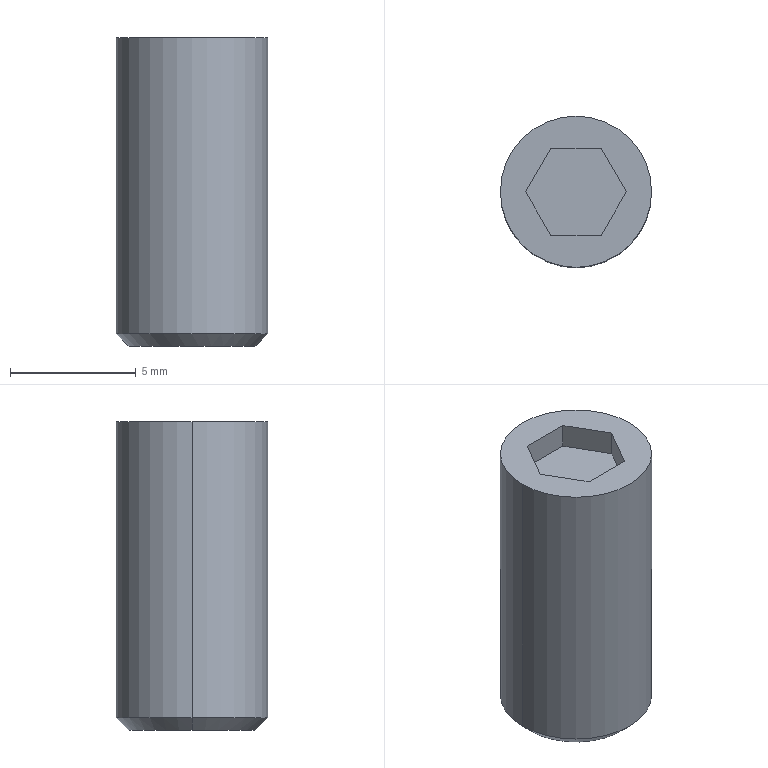Part | SolidWorks | features BaseBody 1 | 1 solid | 13 faces | box 6 x 6 x 12.25 mm | volume 333.743 mm3 | plane 9 | cylinder 2 | cone 2 | commonest cylinder face diameters 6 x2
STEP:
#1=CARTESIAN_POINT('',(24.,133.,18.25));
#2=VERTEX_POINT('',#1);
#3=CARTESIAN_POINT('',(18.,133.,18.25));
#4=VERTEX_POINT('',#3);
#5=CARTESIAN_POINT('',(21.,133.,18.25));
#6=DIRECTION('',(0.,0.,1.));
#7=DIRECTION('',(1.,0.,0.));
#8=AXIS2_PLACEMENT_3D('',#5,#6,#7);
#9=CIRCLE('',#8,3.);
#10=EDGE_CURVE('',#2,#4,#9,.T.);
#11=ORIENTED_EDGE('',*,*,#10,.T.);
#12=CARTESIAN_POINT('',(18.,133.,30.));
#13=VERTEX_POINT('',#12);
#14=CARTESIAN_POINT('',(18.,133.,29.));
#15=DIRECTION('',(0.,0.,1.));
#16=VECTOR('',#15,1000.);
#17=LINE('',#14,#16);
#18=EDGE_CURVE('',#4,#13,#17,.T.);
#19=ORIENTED_EDGE('',*,*,#18,.T.);
#20=CARTESIAN_POINT('',(24.,133.,30.));
#21=VERTEX_POINT('',#20);
#22=CARTESIAN_POINT('',(21.,133.,30.));
#23=DIRECTION('',(0.,0.,-1.));
#24=DIRECTION('',(1.,0.,0.));
#25=AXIS2_PLACEMENT_3D('',#22,#23,#24);
#26=CIRCLE('',#25,3.);
#27=EDGE_CURVE('',#13,#21,#26,.T.);
#28=ORIENTED_EDGE('',*,*,#27,.T.);
#29=CARTESIAN_POINT('',(24.,133.,29.));
#30=DIRECTION('',(0.,0.,1.));
#31=VECTOR('',#30,1000.);
#32=LINE('',#29,#31);
#33=EDGE_CURVE('',#2,#21,#32,.T.);
#34=ORIENTED_EDGE('',*,*,#33,.F.);
#35=EDGE_LOOP('',(#11,#19,#28,#34));
#36=FACE_OUTER_BOUND('',#35,.T.);
#37=CARTESIAN_POINT('',(21.,133.,29.));
#38=DIRECTION('',(0.,0.,1.));
#39=DIRECTION('',(1.,0.,0.));
#40=AXIS2_PLACEMENT_3D('',#37,#38,#39);
#41=CYLINDRICAL_SURFACE('',#40,3.);
#42=ADVANCED_FACE('',(#36),#41,.T.);
#43=CARTESIAN_POINT('',(23.5,133.,17.75));
#44=VERTEX_POINT('',#43);
#45=CARTESIAN_POINT('',(18.5,133.,17.75));
#46=VERTEX_POINT('',#45);
#47=CARTESIAN_POINT('',(21.,133.,17.75));
#48=DIRECTION('',(0.,0.,1.));
#49=DIRECTION('',(1.,0.,0.));
#50=AXIS2_PLACEMENT_3D('',#47,#48,#49);
#51=CIRCLE('',#50,2.5);
#52=EDGE_CURVE('',#44,#46,#51,.T.);
#53=ORIENTED_EDGE('',*,*,#52,.T.);
#54=CARTESIAN_POINT('',(18.,133.,18.25));
#55=DIRECTION('',(-0.7071,0.,0.7071));
#56=VECTOR('',#55,1000.);
#57=LINE('',#54,#56);
#58=EDGE_CURVE('',#46,#4,#57,.T.);
#59=ORIENTED_EDGE('',*,*,#58,.T.);
#60=ORIENTED_EDGE('',*,*,#10,.F.);
#61=CARTESIAN_POINT('',(24.,133.,18.25));
#62=DIRECTION('',(0.7071,0.,0.7071));
#63=VECTOR('',#62,1000.);
#64=LINE('',#61,#63);
#65=EDGE_CURVE('',#44,#2,#64,.T.);
#66=ORIENTED_EDGE('',*,*,#65,.F.);
#67=EDGE_LOOP('',(#53,#59,#60,#66));
#68=FACE_OUTER_BOUND('',#67,.T.);
#69=CARTESIAN_POINT('',(21.,133.,18.25));
#70=DIRECTION('',(0.,0.,1.));
#71=DIRECTION('',(1.,0.,0.));
#72=AXIS2_PLACEMENT_3D('',#69,#70,#71);
#73=CONICAL_SURFACE('',#72,3.,0.7854);
#74=ADVANCED_FACE('',(#68),#73,.T.);
#75=ORIENTED_EDGE('',*,*,#18,.F.);
#76=CARTESIAN_POINT('',(21.,133.,18.25));
#77=DIRECTION('',(0.,0.,1.));
#78=DIRECTION('',(1.,0.,0.));
#79=AXIS2_PLACEMENT_3D('',#76,#77,#78);
#80=CIRCLE('',#79,3.);
#81=EDGE_CURVE('',#4,#2,#80,.T.);
#82=ORIENTED_EDGE('',*,*,#81,.T.);
#83=ORIENTED_EDGE('',*,*,#33,.T.);
#84=CARTESIAN_POINT('',(21.,133.,30.));
#85=DIRECTION('',(0.,0.,-1.));
#86=DIRECTION('',(1.,0.,0.));
#87=AXIS2_PLACEMENT_3D('',#84,#85,#86);
#88=CIRCLE('',#87,3.);
#89=EDGE_CURVE('',#21,#13,#88,.T.);
#90=ORIENTED_EDGE('',*,*,#89,.T.);
#91=EDGE_LOOP('',(#75,#82,#83,#90));
#92=FACE_OUTER_BOUND('',#91,.T.);
#93=CARTESIAN_POINT('',(21.,133.,29.));
#94=DIRECTION('',(0.,0.,1.));
#95=DIRECTION('',(1.,0.,0.));
#96=AXIS2_PLACEMENT_3D('',#93,#94,#95);
#97=CYLINDRICAL_SURFACE('',#96,3.);
#98=ADVANCED_FACE('',(#92),#97,.T.);
#99=ORIENTED_EDGE('',*,*,#89,.F.);
#100=ORIENTED_EDGE('',*,*,#27,.F.);
#101=EDGE_LOOP('',(#99,#100));
#102=FACE_OUTER_BOUND('',#101,.T.);
#103=CARTESIAN_POINT('',(19.,133.,30.));
#104=VERTEX_POINT('',#103);
#105=CARTESIAN_POINT('',(20.,134.732,30.));
#106=VERTEX_POINT('',#105);
#107=CARTESIAN_POINT('',(19.,133.,30.));
#108=DIRECTION('',(0.5,0.866,0.));
#109=VECTOR('',#108,1000.);
#110=LINE('',#107,#109);
#111=EDGE_CURVE('',#104,#106,#110,.T.);
#112=ORIENTED_EDGE('',*,*,#111,.T.);
#113=CARTESIAN_POINT('',(22.,134.732,30.));
#114=VERTEX_POINT('',#113);
#115=CARTESIAN_POINT('',(33.,134.732,30.));
#116=DIRECTION('',(1.,0.,0.));
#117=VECTOR('',#116,1000.);
#118=LINE('',#115,#117);
#119=EDGE_CURVE('',#106,#114,#118,.T.);
#120=ORIENTED_EDGE('',*,*,#119,.T.);
#121=CARTESIAN_POINT('',(23.,133.,30.));
#122=VERTEX_POINT('',#121);
#123=CARTESIAN_POINT('',(22.,134.732,30.));
#124=DIRECTION('',(0.5,-0.866,0.));
#125=VECTOR('',#124,1000.);
#126=LINE('',#123,#125);
#127=EDGE_CURVE('',#114,#122,#126,.T.);
#128=ORIENTED_EDGE('',*,*,#127,.T.);
#129=CARTESIAN_POINT('',(22.,131.268,30.));
#130=VERTEX_POINT('',#129);
#131=CARTESIAN_POINT('',(23.,133.,30.));
#132=DIRECTION('',(-0.5,-0.866,0.));
#133=VECTOR('',#132,1000.);
#134=LINE('',#131,#133);
#135=EDGE_CURVE('',#122,#130,#134,.T.);
#136=ORIENTED_EDGE('',*,*,#135,.T.);
#137=CARTESIAN_POINT('',(20.,131.268,30.));
#138=VERTEX_POINT('',#137);
#139=CARTESIAN_POINT('',(33.,131.268,30.));
#140=DIRECTION('',(-1.,0.,0.));
#141=VECTOR('',#140,1000.);
#142=LINE('',#139,#141);
#143=EDGE_CURVE('',#130,#138,#142,.T.);
#144=ORIENTED_EDGE('',*,*,#143,.T.);
#145=CARTESIAN_POINT('',(20.,131.268,30.));
#146=DIRECTION('',(-0.5,0.866,0.));
#147=VECTOR('',#146,1000.);
#148=LINE('',#145,#147);
#149=EDGE_CURVE('',#138,#104,#148,.T.);
#150=ORIENTED_EDGE('',*,*,#149,.T.);
#151=EDGE_LOOP('',(#112,#120,#128,#136,#144,#150));
#152=FACE_BOUND('',#151,.T.);
#153=CARTESIAN_POINT('',(33.,108.75,30.));
#154=DIRECTION('',(0.,0.,1.));
#155=DIRECTION('',(1.,0.,0.));
#156=AXIS2_PLACEMENT_3D('',#153,#154,#155);
#157=PLANE('',#156);
#158=ADVANCED_FACE('',(#102,#152),#157,.T.);
#159=ORIENTED_EDGE('',*,*,#58,.F.);
#160=CARTESIAN_POINT('',(21.,133.,17.75));
#161=DIRECTION('',(0.,0.,1.));
#162=DIRECTION('',(1.,0.,0.));
#163=AXIS2_PLACEMENT_3D('',#160,#161,#162);
#164=CIRCLE('',#163,2.5);
#165=EDGE_CURVE('',#46,#44,#164,.T.);
#166=ORIENTED_EDGE('',*,*,#165,.T.);
#167=ORIENTED_EDGE('',*,*,#65,.T.);
#168=ORIENTED_EDGE('',*,*,#81,.F.);
#169=EDGE_LOOP('',(#159,#166,#167,#168));
#170=FACE_OUTER_BOUND('',#169,.T.);
#171=CARTESIAN_POINT('',(21.,133.,18.25));
#172=DIRECTION('',(0.,0.,1.));
#173=DIRECTION('',(1.,0.,0.));
#174=AXIS2_PLACEMENT_3D('',#171,#172,#173);
#175=CONICAL_SURFACE('',#174,3.,0.7854);
#176=ADVANCED_FACE('',(#170),#175,.T.);
#177=ORIENTED_EDGE('',*,*,#119,.F.);
#178=CARTESIAN_POINT('',(20.,134.732,29.));
#179=VERTEX_POINT('',#178);
#180=CARTESIAN_POINT('',(20.,134.732,30.));
#181=DIRECTION('',(0.,0.,-1.));
#182=VECTOR('',#181,1000.);
#183=LINE('',#180,#182);
#184=EDGE_CURVE('',#106,#179,#183,.T.);
#185=ORIENTED_EDGE('',*,*,#184,.T.);
#186=CARTESIAN_POINT('',(22.,134.732,29.));
#187=VERTEX_POINT('',#186);
#188=CARTESIAN_POINT('',(20.,134.732,29.));
#189=DIRECTION('',(1.,0.,0.));
#190=VECTOR('',#189,1000.);
#191=LINE('',#188,#190);
#192=EDGE_CURVE('',#179,#187,#191,.T.);
#193=ORIENTED_EDGE('',*,*,#192,.T.);
#194=CARTESIAN_POINT('',(22.,134.732,30.));
#195=DIRECTION('',(0.,0.,1.));
#196=VECTOR('',#195,1000.);
#197=LINE('',#194,#196);
#198=EDGE_CURVE('',#187,#114,#197,.T.);
#199=ORIENTED_EDGE('',*,*,#198,.T.);
#200=EDGE_LOOP('',(#177,#185,#193,#199));
#201=FACE_OUTER_BOUND('',#200,.T.);
#202=CARTESIAN_POINT('',(20.,134.732,30.));
#203=DIRECTION('',(0.,-1.,0.));
#204=DIRECTION('',(0.,0.,-1.));
#205=AXIS2_PLACEMENT_3D('',#202,#203,#204);
#206=PLANE('',#205);
#207=ADVANCED_FACE('',(#201),#206,.T.);
#208=ORIENTED_EDGE('',*,*,#111,.F.);
#209=CARTESIAN_POINT('',(19.,133.,29.));
#210=VERTEX_POINT('',#209);
#211=CARTESIAN_POINT('',(19.,133.,30.));
#212=DIRECTION('',(0.,0.,-1.));
#213=VECTOR('',#212,1000.);
#214=LINE('',#211,#213);
#215=EDGE_CURVE('',#104,#210,#214,.T.);
#216=ORIENTED_EDGE('',*,*,#215,.T.);
#217=CARTESIAN_POINT('',(19.,133.,29.));
#218=DIRECTION('',(0.5,0.866,0.));
#219=VECTOR('',#218,1000.);
#220=LINE('',#217,#219);
#221=EDGE_CURVE('',#210,#179,#220,.T.);
#222=ORIENTED_EDGE('',*,*,#221,.T.);
#223=ORIENTED_EDGE('',*,*,#184,.F.);
#224=EDGE_LOOP('',(#208,#216,#222,#223));
#225=FACE_OUTER_BOUND('',#224,.T.);
#226=CARTESIAN_POINT('',(19.,133.,30.));
#227=DIRECTION('',(0.866,-0.5,0.));
#228=DIRECTION('',(0.5,0.866,0.));
#229=AXIS2_PLACEMENT_3D('',#226,#227,#228);
#230=PLANE('',#229);
#231=ADVANCED_FACE('',(#225),#230,.T.);
#232=ORIENTED_EDGE('',*,*,#149,.F.);
#233=CARTESIAN_POINT('',(20.,131.268,29.));
#234=VERTEX_POINT('',#233);
#235=CARTESIAN_POINT('',(20.,131.268,30.));
#236=DIRECTION('',(0.,0.,-1.));
#237=VECTOR('',#236,1000.);
#238=LINE('',#235,#237);
#239=EDGE_CURVE('',#138,#234,#238,.T.);
#240=ORIENTED_EDGE('',*,*,#239,.T.);
#241=CARTESIAN_POINT('',(20.,131.268,29.));
#242=DIRECTION('',(-0.5,0.866,0.));
#243=VECTOR('',#242,1000.);
#244=LINE('',#241,#243);
#245=EDGE_CURVE('',#234,#210,#244,.T.);
#246=ORIENTED_EDGE('',*,*,#245,.T.);
#247=ORIENTED_EDGE('',*,*,#215,.F.);
#248=EDGE_LOOP('',(#232,#240,#246,#247));
#249=FACE_OUTER_BOUND('',#248,.T.);
#250=CARTESIAN_POINT('',(20.,131.268,30.));
#251=DIRECTION('',(0.866,0.5,0.));
#252=DIRECTION('',(-0.5,0.866,0.));
#253=AXIS2_PLACEMENT_3D('',#250,#251,#252);
#254=PLANE('',#253);
#255=ADVANCED_FACE('',(#249),#254,.T.);
#256=ORIENTED_EDGE('',*,*,#143,.F.);
#257=CARTESIAN_POINT('',(22.,131.268,29.));
#258=VERTEX_POINT('',#257);
#259=CARTESIAN_POINT('',(22.,131.268,30.));
#260=DIRECTION('',(0.,0.,-1.));
#261=VECTOR('',#260,1000.);
#262=LINE('',#259,#261);
#263=EDGE_CURVE('',#130,#258,#262,.T.);
#264=ORIENTED_EDGE('',*,*,#263,.T.);
#265=CARTESIAN_POINT('',(22.,131.268,29.));
#266=DIRECTION('',(-1.,0.,0.));
#267=VECTOR('',#266,1000.);
#268=LINE('',#265,#267);
#269=EDGE_CURVE('',#258,#234,#268,.T.);
#270=ORIENTED_EDGE('',*,*,#269,.T.);
#271=ORIENTED_EDGE('',*,*,#239,.F.);
#272=EDGE_LOOP('',(#256,#264,#270,#271));
#273=FACE_OUTER_BOUND('',#272,.T.);
#274=CARTESIAN_POINT('',(22.,131.268,30.));
#275=DIRECTION('',(0.,1.,0.));
#276=DIRECTION('',(0.,0.,1.));
#277=AXIS2_PLACEMENT_3D('',#274,#275,#276);
#278=PLANE('',#277);
#279=ADVANCED_FACE('',(#273),#278,.T.);
#280=ORIENTED_EDGE('',*,*,#135,.F.);
#281=CARTESIAN_POINT('',(23.,133.,29.));
#282=VERTEX_POINT('',#281);
#283=CARTESIAN_POINT('',(23.,133.,30.));
#284=DIRECTION('',(0.,0.,-1.));
#285=VECTOR('',#284,1000.);
#286=LINE('',#283,#285);
#287=EDGE_CURVE('',#122,#282,#286,.T.);
#288=ORIENTED_EDGE('',*,*,#287,.T.);
#289=CARTESIAN_POINT('',(23.,133.,29.));
#290=DIRECTION('',(-0.5,-0.866,0.));
#291=VECTOR('',#290,1000.);
#292=LINE('',#289,#291);
#293=EDGE_CURVE('',#282,#258,#292,.T.);
#294=ORIENTED_EDGE('',*,*,#293,.T.);
#295=ORIENTED_EDGE('',*,*,#263,.F.);
#296=EDGE_LOOP('',(#280,#288,#294,#295));
#297=FACE_OUTER_BOUND('',#296,.T.);
#298=CARTESIAN_POINT('',(23.,133.,30.));
#299=DIRECTION('',(-0.866,0.5,0.));
#300=DIRECTION('',(-0.5,-0.866,0.));
#301=AXIS2_PLACEMENT_3D('',#298,#299,#300);
#302=PLANE('',#301);
#303=ADVANCED_FACE('',(#297),#302,.T.);
#304=ORIENTED_EDGE('',*,*,#127,.F.);
#305=ORIENTED_EDGE('',*,*,#198,.F.);
#306=CARTESIAN_POINT('',(22.,134.732,29.));
#307=DIRECTION('',(0.5,-0.866,0.));
#308=VECTOR('',#307,1000.);
#309=LINE('',#306,#308);
#310=EDGE_CURVE('',#187,#282,#309,.T.);
#311=ORIENTED_EDGE('',*,*,#310,.T.);
#312=ORIENTED_EDGE('',*,*,#287,.F.);
#313=EDGE_LOOP('',(#304,#305,#311,#312));
#314=FACE_OUTER_BOUND('',#313,.T.);
#315=CARTESIAN_POINT('',(22.,134.732,30.));
#316=DIRECTION('',(-0.866,-0.5,0.));
#317=DIRECTION('',(0.5,-0.866,0.));
#318=AXIS2_PLACEMENT_3D('',#315,#316,#317);
#319=PLANE('',#318);
#320=ADVANCED_FACE('',(#314),#319,.T.);
#321=ORIENTED_EDGE('',*,*,#52,.F.);
#322=ORIENTED_EDGE('',*,*,#165,.F.);
#323=EDGE_LOOP('',(#321,#322));
#324=FACE_OUTER_BOUND('',#323,.T.);
#325=CARTESIAN_POINT('',(55.989,143.,17.75));
#326=DIRECTION('',(0.,0.,-1.));
#327=DIRECTION('',(-1.,0.,0.));
#328=AXIS2_PLACEMENT_3D('',#325,#326,#327);
#329=PLANE('',#328);
#330=ADVANCED_FACE('',(#324),#329,.T.);
#331=ORIENTED_EDGE('',*,*,#293,.F.);
#332=ORIENTED_EDGE('',*,*,#310,.F.);
#333=ORIENTED_EDGE('',*,*,#192,.F.);
#334=ORIENTED_EDGE('',*,*,#221,.F.);
#335=ORIENTED_EDGE('',*,*,#245,.F.);
#336=ORIENTED_EDGE('',*,*,#269,.F.);
#337=EDGE_LOOP('',(#331,#332,#333,#334,#335,#336));
#338=FACE_OUTER_BOUND('',#337,.T.);
#339=CARTESIAN_POINT('',(33.,108.75,29.));
#340=DIRECTION('',(0.,0.,1.));
#341=DIRECTION('',(1.,0.,0.));
#342=AXIS2_PLACEMENT_3D('',#339,#340,#341);
#343=PLANE('',#342);
#344=ADVANCED_FACE('',(#338),#343,.T.);
#345=CLOSED_SHELL('',(#42,#74,#98,#158,#176,#207,#231,#255,#279,#303,#320,#330,#344));
#346=MANIFOLD_SOLID_BREP('',#345);
#347=CARTESIAN_POINT('',(0.,0.,0.));
#348=DIRECTION('',(0.,0.,1.));
#349=DIRECTION('',(1.,0.,0.));
#350=AXIS2_PLACEMENT_3D('',#347,#348,#349);
#351=(LENGTH_UNIT()NAMED_UNIT(*)SI_UNIT(.MILLI.,.METRE.));
#352=UNCERTAINTY_MEASURE_WITH_UNIT(LENGTH_MEASURE(0.00001),#351,'','');
#353=(NAMED_UNIT(*)PLANE_ANGLE_UNIT()SI_UNIT($,.RADIAN.));
#354=(NAMED_UNIT(*)SI_UNIT($,.STERADIAN.)SOLID_ANGLE_UNIT());
#355=(GEOMETRIC_REPRESENTATION_CONTEXT(3)GLOBAL_UNCERTAINTY_ASSIGNED_CONTEXT((#352))GLOBAL_UNIT_ASSIGNED_CONTEXT((#351,#353,#354))REPRESENTATION_CONTEXT('',''));
#356=ADVANCED_BREP_SHAPE_REPRESENTATION('',(#346,#350),#355);